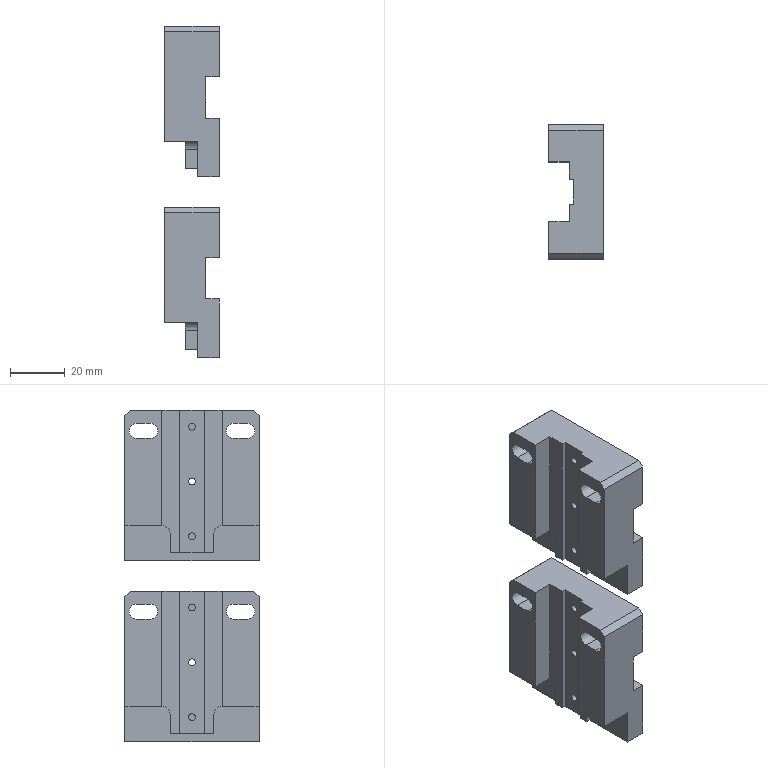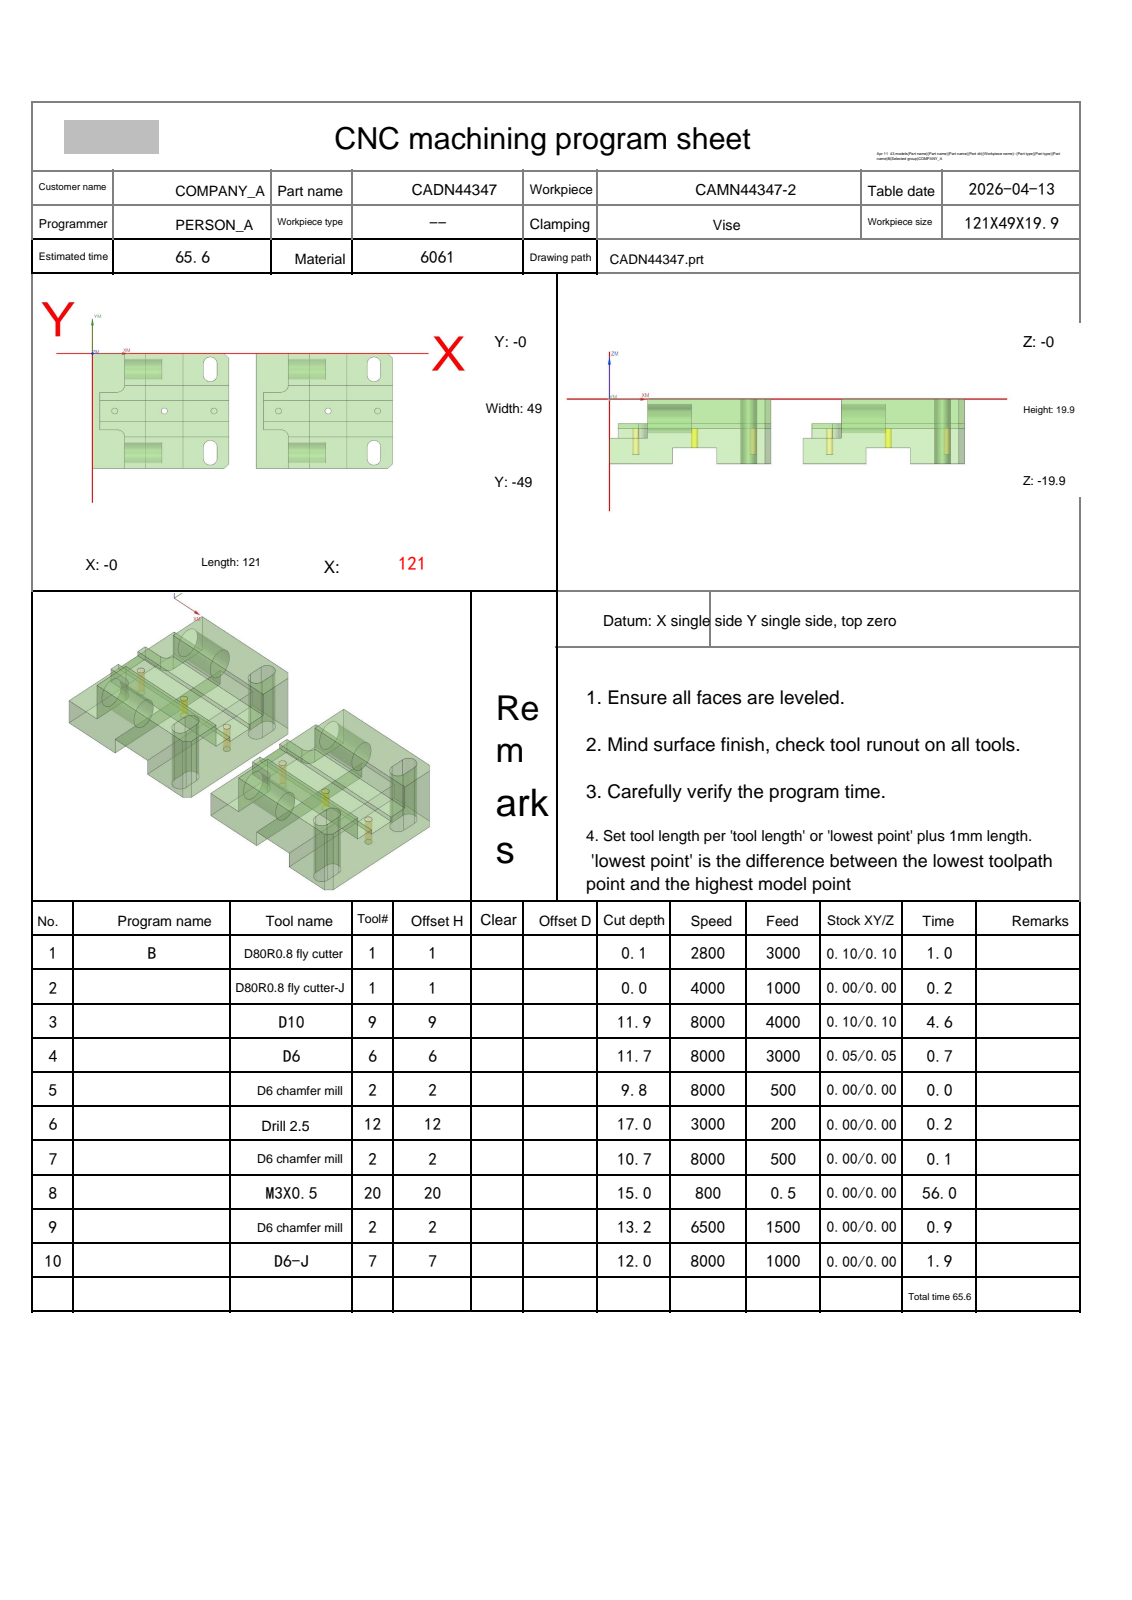NC program | NX | posted by the shop | part box 19.9 x 49 x 121 mm
Lines 5569 to 6263 of 6263:
N5 T02 M06
(D6 chamfer mill  D=6. R=0. H=02 ce=0.00 di=0.05)
G00 G90 G54 X115. Y-24.5 M03 S8000
G43 H02 Z20.
M08
G98 G81 X115. Y-24.5 Z-9.8 R-8. F500.
X75.
X49.
X9.
G80
G00 Z20.
G91 G28 Z0.0
M05
M09
G91 G28 Z0.0
M01
N6 T12 M06
(Drill 2.5 D=2.5 DR_a=118 H=12)
G00 G90 G54 X115. Y-24.5 M03 S3000
G43 H12 Z20.
M08
G98 G83 X115. Y-24.5 Z-17. R-8. F200. Q2.
X75.
X49.
X9.
G80
G00 Z20.
G91 G28 Z0.0
M05
M09
G91 G28 Z0.0
M01
N7 T02 M06
(D6 chamfer mill  D=6. R=0. H=02 ce=0.00 di=0.05)
G00 G90 G54 X9. Y-24.5 M03 S8000
G43 H02 Z20.
M08
G98 G81 X9. Y-24.5 Z-10.75 R-6. F500.
X29.
X49.
X75.
X95.
X115.
G80
G00 Z20.
G91 G28 Z0.0
M05
M09
G91 G28 Z0.0
M01
N8 T20 M06
(M3X0.5 D=2.5 DR_a=180 H=20)
G00 G90 G54 X115. Y-24.5 M03 S800
G43 H20 Z20.
M08
G95
G98 G84 X115. Y-24.5 Z-15. R-8. F.5 Q2.
X75.
X49.
X9.
G80
G94
G00 Z20.
G91 G28 Z0.0
M05
M09
G91 G28 Z0.0
M01
N9 T02 M06
(D6 chamfer mill  D=6. R=0. H=02 ce=0.00 di=0.00)
G00 G90 G54 X34.386 Y-14.727 M03 S6500
G43 H02 Z20.
M08
Z.172
G01 Z-1.199 F1500.
G03 X34.1 Y-14.527 I-1.286 J-1.532
G01 X34.054 Y-14.497
X34. Y-14.5
X13.
G02 X12. Y-13.5 I0.0 J1.
G01 Y0.0
G02 X13. Y1. I1. J0.0
G01 X53.
X53.259 Y.966
X53.5 Y.866
X53.707 Y.707
X55.707 Y-1.293
X55.866 Y-1.5
X55.966 Y-1.741
X56. Y-2.
Y-13.5
G02 X55. Y-14.5 I-1. J0.0
G01 X34.
X33.946 Y-14.497
X33.9 Y-14.527
G03 X33.614 Y-14.727 I1. J-1.732
G01 Z.172
G00 Z10.
X49.023 Y-7.136
Z.172
G01 Z-1.199
G03 X49.223 Y-6.85 I-1.532 J1.286
G01 X49.253 Y-6.804
X49.25 Y-6.75
Y-4.25
G03 X47.5 Y-2.5 I-1.75 J0.0
X45.75 Y-4.25 I0.0 J-1.75
G01 Y-9.25
G03 X47.5 Y-11. I1.75 J0.0
X49.25 Y-9.25 I0.0 J1.75
G01 Y-6.75
X49.253 Y-6.696
X49.223 Y-6.65
G03 X49.023 Y-6.364 I-1.732 J-1.
G01 Z.172
G00 Z10.
X33.614 Y-34.273
Z.172
G01 Z-1.199
G03 X33.9 Y-34.473 I1.286 J1.532
G01 X33.946 Y-34.503
X34. Y-34.5
X55.
G02 X56. Y-35.5 I0.0 J-1.
G01 Y-47.
X55.966 Y-47.259
X55.866 Y-47.5
X55.707 Y-47.707
X53.707 Y-49.707
X53.5 Y-49.866
X53.259 Y-49.966
X53. Y-50.
X13.
G02 X12. Y-49. I0.0 J1.
G01 Y-35.5
G02 X13. Y-34.5 I1. J0.0
G01 X34.
X34.054 Y-34.503
X34.1 Y-34.473
G03 X34.386 Y-34.273 I-1. J1.732
G01 Z.172
G00 Z10.
X49.023 Y-42.636
Z.172
G01 Z-1.199
G03 X49.223 Y-42.35 I-1.532 J1.286
G01 X49.253 Y-42.304
X49.25 Y-42.25
Y-39.75
G03 X47.5 Y-38. I-1.75 J0.0
X45.75 Y-39.75 I0.0 J-1.75
G01 Y-44.75
G03 X47.5 Y-46.5 I1.75 J0.0
X49.25 Y-44.75 I0.0 J1.75
G01 Y-42.25
X49.253 Y-42.196
X49.223 Y-42.15
G03 X49.023 Y-41.864 I-1.732 J-1.
G01 Z.172
G00 Z10.
X99.614 Y-34.273
Z.172
G01 Z-1.199
G03 X99.9 Y-34.473 I1.286 J1.532
G01 X99.946 Y-34.503
X100. Y-34.5
X121.
G02 X122. Y-35.5 I0.0 J-1.
G01 Y-47.
X121.966 Y-47.259
X121.866 Y-47.5
X121.707 Y-47.707
X119.707 Y-49.707
X119.5 Y-49.866
X119.259 Y-49.966
X119. Y-50.
X79.
G02 X78. Y-49. I0.0 J1.
G01 Y-35.5
G02 X79. Y-34.5 I1. J0.0
G01 X100.
X100.054 Y-34.503
X100.1 Y-34.473
G03 X100.386 Y-34.273 I-1. J1.732
G01 Z.172
G00 Z10.
X115.023 Y-42.636
Z.172
G01 Z-1.199
G03 X115.223 Y-42.35 I-1.532 J1.286
G01 X115.253 Y-42.304
X115.25 Y-42.25
Y-39.75
G03 X113.5 Y-38. I-1.75 J0.0
X111.75 Y-39.75 I0.0 J-1.75
G01 Y-44.75
G03 X113.5 Y-46.5 I1.75 J0.0
X115.25 Y-44.75 I0.0 J1.75
G01 Y-42.25
X115.253 Y-42.196
X115.223 Y-42.15
G03 X115.023 Y-41.864 I-1.732 J-1.
G01 Z.172
G00 Z10.
X100.386 Y-14.727
Z.172
G01 Z-1.199
G03 X100.1 Y-14.527 I-1.286 J-1.532
G01 X100.054 Y-14.497
X100. Y-14.5
X79.
G02 X78. Y-13.5 I0.0 J1.
G01 Y0.0
G02 X79. Y1. I1. J0.0
G01 X119.
X119.259 Y.966
X119.5 Y.866
X119.707 Y.707
X121.707 Y-1.293
X121.866 Y-1.5
X121.966 Y-1.741
X122. Y-2.
Y-13.5
G02 X121. Y-14.5 I-1. J0.0
G01 X100.
X99.946 Y-14.497
X99.9 Y-14.527
G03 X99.614 Y-14.727 I1. J-1.732
G01 Z.172
G00 Z10.
X115.023 Y-7.136
Z.172
G01 Z-1.199
G03 X115.223 Y-6.85 I-1.532 J1.286
G01 X115.253 Y-6.804
X115.25 Y-6.75
Y-4.25
G03 X113.5 Y-2.5 I-1.75 J0.0
X111.75 Y-4.25 I0.0 J-1.75
G01 Y-9.25
G03 X113.5 Y-11. I1.75 J0.0
X115.25 Y-9.25 I0.0 J1.75
G01 Y-6.75
X115.253 Y-6.696
X115.223 Y-6.65
G03 X115.023 Y-6.364 I-1.732 J-1.
G01 Z.172
G00 Z10.
X76.414 Y-33.586
Z-1.819
G01 Z-8.699
X76.361 Y-33.541
X76.341 Y-33.534
X76. Y-33.5
X69.
G02 X68. Y-32.5 I0.0 J1.
G01 Y-29.05
G02 X69. Y-28.05 I1. J0.0
G01 X121.
G02 X122. Y-29.05 I0.0 J-1.
G01 Y-32.376
X122.008 Y-32.406
X122.068 Y-32.491
Z-1.794
G00 Z10.
Y-16.509
Z-1.794
G01 Z-8.699
X122.008 Y-16.594
X122. Y-16.624
Y-19.95
G02 X121. Y-20.95 I-1. J0.0
G01 X69.
G02 X68. Y-19.95 I0.0 J1.
G01 Y-16.5
G02 X69. Y-15.5 I1. J0.0
G01 X76.
X76.341 Y-15.466
X76.368 Y-15.459
X76.386 Y-15.448
X76.43 Y-15.395
Z-1.794
G00 Z10.
X10.414 Y-33.586
Z-1.819
G01 Z-8.699
X10.361 Y-33.541
X10.341 Y-33.534
X10. Y-33.5
X3.
G02 X2. Y-32.5 I0.0 J1.
G01 Y-29.05
G02 X3. Y-28.05 I1. J0.0
G01 X55.
G02 X56. Y-29.05 I0.0 J-1.
G01 Y-32.376
X56.008 Y-32.406
X56.068 Y-32.491
Z-1.794
G00 Z10.
Y-16.509
Z-1.794
G01 Z-8.699
X56.008 Y-16.594
X56. Y-16.624
Y-19.95
G02 X55. Y-20.95 I-1. J0.0
G01 X3.
G02 X2. Y-19.95 I0.0 J1.
G01 Y-16.5
G02 X3. Y-15.5 I1. J0.0
G01 X10.
X10.341 Y-15.466
X10.368 Y-15.459
X10.386 Y-15.448
X10.43 Y-15.395
Z-1.794
G00 Z10.
X2. Y-26.562
Z-6.199
G01 Z-10.199
Y-22.438
Z-6.199
G00 Z10.
X56.
Z-6.199
G01 Z-10.199
Y-26.562
Z-6.199
G00 Z10.
X68.
Z-6.199
G01 Z-10.199
Y-22.438
Z-6.199
G00 Z10.
X122.
Z-6.199
G01 Z-10.199
Y-26.562
Z-6.199
G00 Z10.
X75.993 Y-50.068
Z-1.793
G01 Z-13.199
X75.907 Y-50.008
X75.877 Y-50.
X66.
G02 X65. Y-49. I0.0 J1.
G01 Y0.0
G02 X66. Y1. I1. J0.0
G01 X75.877
X75.907 Y1.008
X75.993 Y1.068
Z-1.793
G00 Z10.
X9.993 Y-50.068
Z-1.793
G01 Z-13.199
X9.907 Y-50.008
X9.877 Y-50.
X0.0
G02 X-1. Y-49. I0.0 J1.
G01 Y0.0
G02 X0.0 Y1. I1. J0.0
G01 X9.877
X9.907 Y1.008
X9.993 Y1.068
Z-1.793
G00 Z20.
G91 G28 Z0.0
M05
M09
G91 G28 Z0.0
M01
N10 T07 M06
(D6-J  D=6. R=0. H=07 ce=0.40 di=0.00)
G00 G90 G54 X-1.2 Y-25.7 M03 S8000
G43 H07 Z14.902
M08
Z-6.
G01 Z-7.5 F1000.
X1.2
G03 X2.4 Y-24.5 I0.0 J1.2
G01 Y-17.498
G02 X2.998 Y-16.9 I.6 J-.002
G01 X55.002
G02 X55.6 Y-17.498 I-.002 J-.6
G01 Y-31.502
G02 X55.002 Y-32.1 I-.6 J.002
G01 X2.998
G02 X2.4 Y-31.502 I.002 J.6
G01 Y-23.263
G02 X2.593 Y-22.822 I.6 J0.0
G01 X5.594 Y-20.058
G02 X6. Y-19.9 I.406 J-.442
G01 X52.002
G02 X52.6 Y-20.498 I-.002 J-.6
G01 Y-28.502
G02 X52.002 Y-29.1 I-.6 J.002
G01 X5.998
G02 X5.4 Y-28.502 I.002 J.6
G01 Y-23.578
G02 X5.94 Y-23.038 I.54 J0.0
G01 X5.977 Y-23.039
X8.178 Y-23.188
X8.218 Y-23.19
G03 X8.609 Y-23.045 I0.0 J.6
G02 X8.998 Y-22.9 I.391 J-.455
G01 X49.002
G02 X49.6 Y-23.498 I-.002 J-.6
G01 Y-25.502
G02 X49.002 Y-26.1 I-.6 J.002
G01 X8.998
G02 X8.4 Y-25.502 I.002 J.6
G01 Y-23.498
G02 X8.476 Y-23.209 I.6 J-.002
X8.998 Y-22.9 I.524 J-.291
G01 X9.362
G03 X10.562 Y-21.7 I0.0 J1.2
G01 Z-6.
G00 Z-3.5
X125.2 Y-23.3
Z-6.
G01 Z-7.5
X122.8
G03 X121.6 Y-24.5 I0.0 J-1.2
G01 Y-31.502
G02 X121.002 Y-32.1 I-.6 J.002
G01 X68.998
G02 X68.4 Y-31.502 I.002 J.6
G01 Y-17.498
G02 X68.998 Y-16.9 I.6 J-.002
G01 X121.002
G02 X121.6 Y-17.498 I-.002 J-.6
G01 Y-27.5
G02 X121.18 Y-28.072 I-.6 J0.0
G01 X118.507 Y-28.912
X118.418 Y-28.937
X118.344 Y-28.992
G02 X118.002 Y-29.1 I-.344 J.492
G01 X71.998
G02 X71.4 Y-28.502 I.002 J.6
G01 Y-20.498
G02 X71.998 Y-19.9 I.6 J-.002
G01 X118.002
G02 X118.6 Y-20.498 I-.002 J-.6
G01 Y-25.422
G02 X118.06 Y-25.962 I-.54 J0.0
G01 X118.023 Y-25.961
X115.822 Y-25.812
X115.782 Y-25.81
G03 X115.391 Y-25.955 I0.0 J-.6
G02 X115.002 Y-26.1 I-.391 J.455
G01 X74.998
G02 X74.4 Y-25.502 I.002 J.6
G01 Y-23.498
G02 X74.998 Y-22.9 I.6 J-.002
G01 X115.002
G02 X115.6 Y-23.498 I-.002 J-.6
G01 Y-25.502
G02 X115.524 Y-25.791 I-.6 J.002
X115.002 Y-26.1 I-.524 J.291
G01 X114.638
G03 X113.438 Y-27.3 I0.0 J-1.2
G01 Z-6.
G00 Z14.902
G00 G90 X-1.2 Y-31.1 M03 S8000
Z14.902
Z-6.5
G01 Z-7.5 F1000.
G41 D07
Y-31.3
G03 X0.0 Y-32.5 I1.2 J0.0
G01 X58.
G03 X59.2 Y-31.3 I0.0 J1.2
G01 G40 Y-31.1
Z-6.5
G00 Y-17.9
G01 Z-7.5
G41 D07
Y-17.7
G03 X58. Y-16.5 I-1.2 J0.0
G01 X0.0
G03 X-1.2 Y-17.7 I0.0 J-1.2
G01 G40 Y-17.9
Z-6.5
G00 Z-2.5
X64.8 Y-31.1
Z-6.5
G01 Z-7.5
G41 D07
Y-31.3
G03 X66. Y-32.5 I1.2 J0.0
G01 X124.
G03 X125.2 Y-31.3 I0.0 J1.2
G01 G40 Y-31.1
Z-6.5
G00 Y-17.9
G01 Z-7.5
G41 D07
Y-17.7
G03 X124. Y-16.5 I-1.2 J0.0
G01 X66.
G03 X64.8 Y-17.7 I0.0 J-1.2
G01 G40 Y-17.9
Z-6.5
G00 Z14.902
G00 G90 X-4.2 Y-43.95 M03 S8000
Z14.902
Z-10.5
G01 Z-12. F1000.
X-1.8
G03 X-.6 Y-42.75 I0.0 J1.2
G01 Y.002
G02 X-.002 Y.6 I.6 J-.002
G01 X9.002
G02 X9.6 Y.002 I-.002 J-.6
G01 Y-12.502
G02 X9.002 Y-13.1 I-.6 J.002
G01 X2.998
G02 X2.398 Y-12.5 I0.0 J.6
G01 X2.417 Y-12.35
X2.866 Y-10.613
X2.885 Y-10.463
G03 X2.642 Y-9.982 I-.6 J0.0
G02 X2.4 Y-9.502 I.358 J.482
G01 Y-2.998
G02 X2.998 Y-2.4 I.6 J-.002
G01 X6.002
G02 X6.6 Y-2.998 I-.002 J-.6
G01 Y-9.502
G02 X6.002 Y-10.1 I-.6 J.002
G01 X4.92
G03 X4.356 Y-10.497 I0.0 J-.6
G01 X3.563 Y-12.703
G02 X2.998 Y-13.1 I-.565 J.203
G01 X-.4
Y-35.9
X9.002
G02 X9.6 Y-36.498 I-.002 J-.6
G01 Y-49.002
G02 X9.002 Y-49.6 I-.6 J.002
G01 X-.002
G02 X-.6 Y-49. I.002 J.6
G01 Y-39.75
G02 X0.0 Y-39.15 I.6 J0.0
G01 X.088 Y-39.156
X1.915 Y-39.427
X2.002 Y-39.433
G03 X2.501 Y-39.167 I0.0 J.6
G02 X2.998 Y-38.9 I.499 J-.333
G01 X6.002
G02 X6.6 Y-39.498 I-.002 J-.6
G01 Y-46.002
G02 X6.002 Y-46.6 I-.6 J.002
G01 X2.998
G02 X2.4 Y-46.002 I.002 J.6
G01 Y-39.75
Y-39.498
G02 X2.811 Y-38.931 I.6 J-.002
G03 X3.632 Y-37.792 I-.378 J1.139
X3.571 Y-37.413 I-1.2 J0.0
G01 Z-10.5
G00 Z14.902
X61.8 Y-43.95
Z-10.5
G01 Z-12.
X64.2
G03 X65.4 Y-42.75 I0.0 J1.2
G01 Y.002
G02 X65.998 Y.6 I.6 J-.002
G01 X75.002
G02 X75.6 Y.002 I-.002 J-.6
G01 Y-12.502
G02 X75.002 Y-13.1 I-.6 J.002
G01 X68.998
G02 X68.398 Y-12.5 I0.0 J.6
G01 X68.417 Y-12.35
X68.866 Y-10.613
X68.885 Y-10.464
G03 X68.642 Y-9.982 I-.6 J0.0
G02 X68.4 Y-9.502 I.358 J.482
G01 Y-2.998
G02 X68.998 Y-2.4 I.6 J-.002
G01 X72.002
G02 X72.6 Y-2.998 I-.002 J-.6
G01 Y-9.502
G02 X72.002 Y-10.1 I-.6 J.002
G01 X70.92
G03 X70.356 Y-10.497 I0.0 J-.6
G01 X69.563 Y-12.703
G02 X68.998 Y-13.1 I-.565 J.203
G01 X65.6
Y-35.9
X75.002
G02 X75.6 Y-36.498 I-.002 J-.6
G01 Y-49.002
G02 X75.002 Y-49.6 I-.6 J.002
G01 X65.998
G02 X65.4 Y-49. I.002 J.6
G01 Y-39.75
G02 X66. Y-39.15 I.6 J0.0
G01 X66.088 Y-39.156
X67.915 Y-39.427
X68.002 Y-39.433
G03 X68.501 Y-39.167 I0.0 J.6
G02 X68.998 Y-38.9 I.499 J-.333
G01 X72.002
G02 X72.6 Y-39.498 I-.002 J-.6
G01 Y-46.002
G02 X72.002 Y-46.6 I-.6 J.002
G01 X68.998
G02 X68.4 Y-46.002 I.002 J.6
G01 Y-39.75
Y-39.498
G02 X68.811 Y-38.931 I.6 J-.002
G03 X69.632 Y-37.792 I-.378 J1.139
X69.571 Y-37.413 I-1.2 J0.0
G01 Z-10.5
G00 Z14.902
G00 G90 X-1.2 Y-24.651 M03 S8000
Z14.902
Z-8.
G01 Z-9. F1000.
G41 D07
Y-24.851
G03 X0.0 Y-26.05 I1.2 J.001
G01 X58.
G03 X59.2 Y-24.851 I0.0 J1.2
G01 G40 Y-24.651
Y-24.349
G41 D07
Y-24.149
G03 X58. Y-22.95 I-1.2 J-.001
G01 X0.0
G03 X-1.2 Y-24.149 I0.0 J-1.2
G01 G40 Y-24.349
Z-8.
G00 Z3.
X64.8 Y-24.65
Z-8.
G01 Z-9.
G41 D07
Y-24.85
G03 X66. Y-26.05 I1.2 J0.0
G01 X124.
G03 X125.2 Y-24.851 I0.0 J1.2
G01 G40 Y-24.651
Y-24.35
G41 D07
Y-24.15
G03 X124. Y-22.95 I-1.2 J-.001
G01 X66.
G03 X64.8 Y-24.15 I0.0 J-1.2
G01 G40 Y-24.35
Z-8.
G00 Z14.902
G00 G90 X8.601 Y-53.2 M03 S8000
Z14.902
Z-11.
G01 Z-12. F1000.
G41 D07
X8.801
G03 X10. Y-52. I-.001 J1.2
G01 Y-35.5
X0.0
Y-13.5
X10.
Y3.
G03 X8.8 Y4.2 I-1.2 J0.0
G01 G40 X8.6
Z-11.
G00 Z14.902
X74.601 Y-53.2
Z-11.
G01 Z-12.
G41 D07
X74.801
G03 X76. Y-52. I-.001 J1.2
G01 Y-35.5
X66.
Y-13.5
X76.
Y3.
G03 X74.801 Y4.2 I-1.2 J0.0
G01 G40 X74.601
Z-11.
G00 Z14.902
M05
M09
G91 G28 Z0.0
G91 G28 Y0.0
M30
%